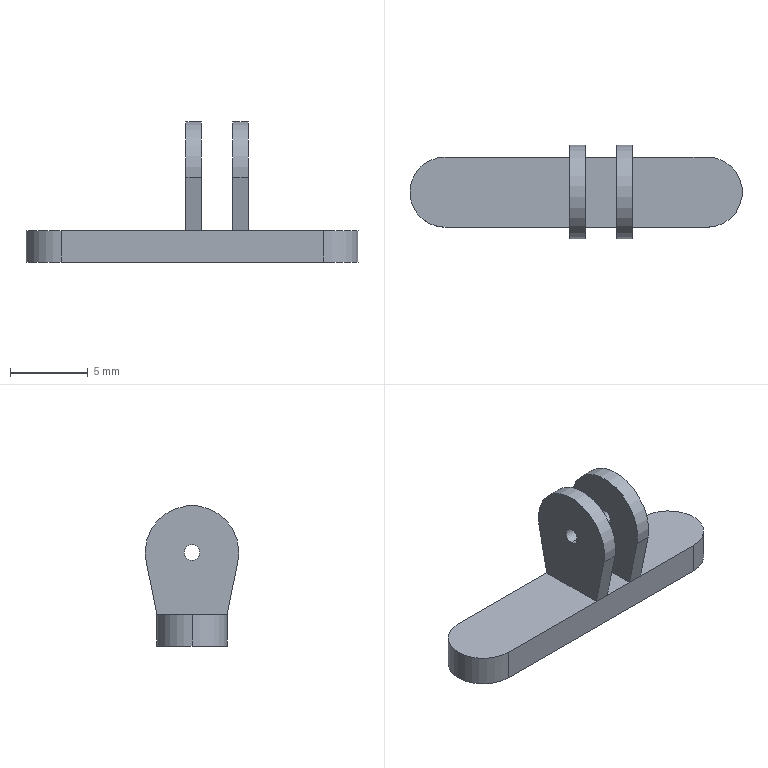Part | SolidWorks | features ICE 2, Extrusion 1 | 1 solid | 21 faces | box 21.3 x 6 x 9 mm | volume 252.148 mm3 | plane 12 | cylinder 9 | commonest cylinder face diameters 1 x4 4.5 x3 6 x2
STEP:
#1=CARTESIAN_POINT('',(8.,0.0009773,5.5));
#2=VERTEX_POINT('',#1);
#3=CARTESIAN_POINT('',(8.,0.0009773,6.5));
#4=VERTEX_POINT('',#3);
#5=CARTESIAN_POINT('',(8.,0.0009773,6.));
#6=DIRECTION('',(-1.,0.,0.));
#7=DIRECTION('',(0.,0.,1.));
#8=AXIS2_PLACEMENT_3D('',#5,#6,#7);
#9=CIRCLE('',#8,0.5);
#10=EDGE_CURVE('',#2,#4,#9,.T.);
#11=ORIENTED_EDGE('',*,*,#10,.T.);
#12=CARTESIAN_POINT('',(9.,0.0009773,6.5));
#13=VERTEX_POINT('',#12);
#14=CARTESIAN_POINT('',(8.,0.0009773,6.5));
#15=DIRECTION('',(1.,0.,0.));
#16=VECTOR('',#15,1000.);
#17=LINE('',#14,#16);
#18=EDGE_CURVE('',#4,#13,#17,.T.);
#19=ORIENTED_EDGE('',*,*,#18,.T.);
#20=CARTESIAN_POINT('',(9.,0.0009773,5.5));
#21=VERTEX_POINT('',#20);
#22=CARTESIAN_POINT('',(9.,0.0009773,6.));
#23=DIRECTION('',(-1.,0.,0.));
#24=DIRECTION('',(0.,0.,1.));
#25=AXIS2_PLACEMENT_3D('',#22,#23,#24);
#26=CIRCLE('',#25,0.5);
#27=EDGE_CURVE('',#21,#13,#26,.T.);
#28=ORIENTED_EDGE('',*,*,#27,.F.);
#29=CARTESIAN_POINT('',(8.,0.0009773,5.5));
#30=DIRECTION('',(1.,0.,0.));
#31=VECTOR('',#30,1000.);
#32=LINE('',#29,#31);
#33=EDGE_CURVE('',#2,#21,#32,.T.);
#34=ORIENTED_EDGE('',*,*,#33,.F.);
#35=EDGE_LOOP('',(#11,#19,#28,#34));
#36=FACE_OUTER_BOUND('',#35,.T.);
#37=CARTESIAN_POINT('',(8.,0.0009773,6.));
#38=DIRECTION('',(1.,0.,0.));
#39=DIRECTION('',(0.,0.,-1.));
#40=AXIS2_PLACEMENT_3D('',#37,#38,#39);
#41=CYLINDRICAL_SURFACE('',#40,0.5);
#42=ADVANCED_FACE('',(#36),#41,.F.);
#43=CARTESIAN_POINT('',(-2.25,0.,2.));
#44=VERTEX_POINT('',#43);
#45=CARTESIAN_POINT('',(0.,-2.25,2.));
#46=VERTEX_POINT('',#45);
#47=CARTESIAN_POINT('',(0.,0.,2.));
#48=DIRECTION('',(0.,0.,1.));
#49=DIRECTION('',(1.,0.,0.));
#50=AXIS2_PLACEMENT_3D('',#47,#48,#49);
#51=CIRCLE('',#50,2.25);
#52=EDGE_CURVE('',#44,#46,#51,.T.);
#53=ORIENTED_EDGE('',*,*,#52,.F.);
#54=CARTESIAN_POINT('',(-2.25,0.,0.));
#55=VERTEX_POINT('',#54);
#56=CARTESIAN_POINT('',(-2.25,0.,2.));
#57=DIRECTION('',(0.,0.,-1.));
#58=VECTOR('',#57,1000.);
#59=LINE('',#56,#58);
#60=EDGE_CURVE('',#44,#55,#59,.T.);
#61=ORIENTED_EDGE('',*,*,#60,.T.);
#62=CARTESIAN_POINT('',(0.,-2.25,0.));
#63=VERTEX_POINT('',#62);
#64=CARTESIAN_POINT('',(0.,0.,0.));
#65=DIRECTION('',(0.,0.,1.));
#66=DIRECTION('',(1.,0.,0.));
#67=AXIS2_PLACEMENT_3D('',#64,#65,#66);
#68=CIRCLE('',#67,2.25);
#69=EDGE_CURVE('',#55,#63,#68,.T.);
#70=ORIENTED_EDGE('',*,*,#69,.T.);
#71=CARTESIAN_POINT('',(0.,-2.25,2.));
#72=DIRECTION('',(0.,0.,-1.));
#73=VECTOR('',#72,1000.);
#74=LINE('',#71,#73);
#75=EDGE_CURVE('',#46,#63,#74,.T.);
#76=ORIENTED_EDGE('',*,*,#75,.F.);
#77=EDGE_LOOP('',(#53,#61,#70,#76));
#78=FACE_OUTER_BOUND('',#77,.T.);
#79=CARTESIAN_POINT('',(0.,0.,2.));
#80=DIRECTION('',(0.,0.,-1.));
#81=DIRECTION('',(-1.,0.,0.));
#82=AXIS2_PLACEMENT_3D('',#79,#80,#81);
#83=CYLINDRICAL_SURFACE('',#82,2.25);
#84=ADVANCED_FACE('',(#78),#83,.T.);
#85=CARTESIAN_POINT('',(11.,0.0009773,6.5));
#86=VERTEX_POINT('',#85);
#87=CARTESIAN_POINT('',(11.,0.0009773,5.5));
#88=VERTEX_POINT('',#87);
#89=CARTESIAN_POINT('',(11.,0.0009773,6.));
#90=DIRECTION('',(1.,0.,0.));
#91=DIRECTION('',(0.,0.,-1.));
#92=AXIS2_PLACEMENT_3D('',#89,#90,#91);
#93=CIRCLE('',#92,0.5);
#94=EDGE_CURVE('',#86,#88,#93,.T.);
#95=ORIENTED_EDGE('',*,*,#94,.F.);
#96=CARTESIAN_POINT('',(12.,0.0009773,6.5));
#97=VERTEX_POINT('',#96);
#98=CARTESIAN_POINT('',(8.,0.0009773,6.5));
#99=DIRECTION('',(1.,0.,0.));
#100=VECTOR('',#99,1000.);
#101=LINE('',#98,#100);
#102=EDGE_CURVE('',#86,#97,#101,.T.);
#103=ORIENTED_EDGE('',*,*,#102,.T.);
#104=CARTESIAN_POINT('',(12.,0.0009773,5.5));
#105=VERTEX_POINT('',#104);
#106=CARTESIAN_POINT('',(12.,0.0009773,6.));
#107=DIRECTION('',(-1.,0.,0.));
#108=DIRECTION('',(0.,0.,1.));
#109=AXIS2_PLACEMENT_3D('',#106,#107,#108);
#110=CIRCLE('',#109,0.5);
#111=EDGE_CURVE('',#105,#97,#110,.T.);
#112=ORIENTED_EDGE('',*,*,#111,.F.);
#113=CARTESIAN_POINT('',(8.,0.0009773,5.5));
#114=DIRECTION('',(1.,0.,0.));
#115=VECTOR('',#114,1000.);
#116=LINE('',#113,#115);
#117=EDGE_CURVE('',#88,#105,#116,.T.);
#118=ORIENTED_EDGE('',*,*,#117,.F.);
#119=EDGE_LOOP('',(#95,#103,#112,#118));
#120=FACE_OUTER_BOUND('',#119,.T.);
#121=CARTESIAN_POINT('',(8.,0.0009773,6.));
#122=DIRECTION('',(1.,0.,0.));
#123=DIRECTION('',(0.,0.,-1.));
#124=AXIS2_PLACEMENT_3D('',#121,#122,#123);
#125=CYLINDRICAL_SURFACE('',#124,0.5);
#126=ADVANCED_FACE('',(#120),#125,.F.);
#127=CARTESIAN_POINT('',(11.,2.25,2.));
#128=VERTEX_POINT('',#127);
#129=CARTESIAN_POINT('',(12.,2.25,2.));
#130=VERTEX_POINT('',#129);
#131=CARTESIAN_POINT('',(8.,2.25,2.));
#132=DIRECTION('',(1.,0.,0.));
#133=VECTOR('',#132,1000.);
#134=LINE('',#131,#133);
#135=EDGE_CURVE('',#128,#130,#134,.T.);
#136=ORIENTED_EDGE('',*,*,#135,.F.);
#137=CARTESIAN_POINT('',(11.,2.941,5.403));
#138=VERTEX_POINT('',#137);
#139=CARTESIAN_POINT('',(11.,2.25,2.));
#140=DIRECTION('',(0.,0.199,0.98));
#141=VECTOR('',#140,1000.);
#142=LINE('',#139,#141);
#143=EDGE_CURVE('',#128,#138,#142,.T.);
#144=ORIENTED_EDGE('',*,*,#143,.T.);
#145=CARTESIAN_POINT('',(12.,2.941,5.403));
#146=VERTEX_POINT('',#145);
#147=CARTESIAN_POINT('',(8.,2.941,5.403));
#148=DIRECTION('',(1.,0.,0.));
#149=VECTOR('',#148,1000.);
#150=LINE('',#147,#149);
#151=EDGE_CURVE('',#138,#146,#150,.T.);
#152=ORIENTED_EDGE('',*,*,#151,.T.);
#153=CARTESIAN_POINT('',(12.,2.25,2.));
#154=DIRECTION('',(0.,-0.199,-0.98));
#155=VECTOR('',#154,1000.);
#156=LINE('',#153,#155);
#157=EDGE_CURVE('',#146,#130,#156,.T.);
#158=ORIENTED_EDGE('',*,*,#157,.T.);
#159=EDGE_LOOP('',(#136,#144,#152,#158));
#160=FACE_OUTER_BOUND('',#159,.T.);
#161=CARTESIAN_POINT('',(8.,2.25,2.));
#162=DIRECTION('',(0.,-0.98,0.199));
#163=DIRECTION('',(0.,-0.199,-0.98));
#164=AXIS2_PLACEMENT_3D('',#161,#162,#163);
#165=PLANE('',#164);
#166=ADVANCED_FACE('',(#160),#165,.F.);
#167=CARTESIAN_POINT('',(11.,-2.939,5.404));
#168=VERTEX_POINT('',#167);
#169=CARTESIAN_POINT('',(12.,-2.939,5.404));
#170=VERTEX_POINT('',#169);
#171=CARTESIAN_POINT('',(8.,-2.939,5.404));
#172=DIRECTION('',(1.,0.,0.));
#173=VECTOR('',#172,1000.);
#174=LINE('',#171,#173);
#175=EDGE_CURVE('',#168,#170,#174,.T.);
#176=ORIENTED_EDGE('',*,*,#175,.F.);
#177=CARTESIAN_POINT('',(11.,-2.249,2.));
#178=VERTEX_POINT('',#177);
#179=CARTESIAN_POINT('',(11.,-2.249,2.));
#180=DIRECTION('',(0.,0.1987,-0.9801));
#181=VECTOR('',#180,1000.);
#182=LINE('',#179,#181);
#183=EDGE_CURVE('',#168,#178,#182,.T.);
#184=ORIENTED_EDGE('',*,*,#183,.T.);
#185=CARTESIAN_POINT('',(12.,-2.249,2.));
#186=VERTEX_POINT('',#185);
#187=CARTESIAN_POINT('',(8.,-2.249,2.));
#188=DIRECTION('',(1.,0.,0.));
#189=VECTOR('',#188,1000.);
#190=LINE('',#187,#189);
#191=EDGE_CURVE('',#178,#186,#190,.T.);
#192=ORIENTED_EDGE('',*,*,#191,.T.);
#193=CARTESIAN_POINT('',(12.,-2.249,2.));
#194=DIRECTION('',(0.,-0.1987,0.9801));
#195=VECTOR('',#194,1000.);
#196=LINE('',#193,#195);
#197=EDGE_CURVE('',#186,#170,#196,.T.);
#198=ORIENTED_EDGE('',*,*,#197,.T.);
#199=EDGE_LOOP('',(#176,#184,#192,#198));
#200=FACE_OUTER_BOUND('',#199,.T.);
#201=CARTESIAN_POINT('',(8.,-2.249,2.));
#202=DIRECTION('',(0.,0.9801,0.1987));
#203=DIRECTION('',(0.,-0.1987,0.9801));
#204=AXIS2_PLACEMENT_3D('',#201,#202,#203);
#205=PLANE('',#204);
#206=ADVANCED_FACE('',(#200),#205,.F.);
#207=CARTESIAN_POINT('',(8.,-2.939,5.404));
#208=VERTEX_POINT('',#207);
#209=CARTESIAN_POINT('',(9.,-2.939,5.404));
#210=VERTEX_POINT('',#209);
#211=CARTESIAN_POINT('',(8.,-2.939,5.404));
#212=DIRECTION('',(1.,0.,0.));
#213=VECTOR('',#212,1000.);
#214=LINE('',#211,#213);
#215=EDGE_CURVE('',#208,#210,#214,.T.);
#216=ORIENTED_EDGE('',*,*,#215,.T.);
#217=CARTESIAN_POINT('',(9.,2.941,5.403));
#218=VERTEX_POINT('',#217);
#219=CARTESIAN_POINT('',(9.,0.0009773,6.));
#220=DIRECTION('',(-1.,0.,0.));
#221=DIRECTION('',(0.,0.,1.));
#222=AXIS2_PLACEMENT_3D('',#219,#220,#221);
#223=CIRCLE('',#222,3.);
#224=EDGE_CURVE('',#210,#218,#223,.T.);
#225=ORIENTED_EDGE('',*,*,#224,.T.);
#226=CARTESIAN_POINT('',(8.,2.941,5.403));
#227=VERTEX_POINT('',#226);
#228=CARTESIAN_POINT('',(8.,2.941,5.403));
#229=DIRECTION('',(1.,0.,0.));
#230=VECTOR('',#229,1000.);
#231=LINE('',#228,#230);
#232=EDGE_CURVE('',#227,#218,#231,.T.);
#233=ORIENTED_EDGE('',*,*,#232,.F.);
#234=CARTESIAN_POINT('',(8.,0.0009773,6.));
#235=DIRECTION('',(-1.,0.,0.));
#236=DIRECTION('',(0.,0.,1.));
#237=AXIS2_PLACEMENT_3D('',#234,#235,#236);
#238=CIRCLE('',#237,3.);
#239=EDGE_CURVE('',#208,#227,#238,.T.);
#240=ORIENTED_EDGE('',*,*,#239,.F.);
#241=EDGE_LOOP('',(#216,#225,#233,#240));
#242=FACE_OUTER_BOUND('',#241,.T.);
#243=CARTESIAN_POINT('',(8.,0.0009773,6.));
#244=DIRECTION('',(1.,0.,0.));
#245=DIRECTION('',(0.,0.,-1.));
#246=AXIS2_PLACEMENT_3D('',#243,#244,#245);
#247=CYLINDRICAL_SURFACE('',#246,3.);
#248=ADVANCED_FACE('',(#242),#247,.T.);
#249=ORIENTED_EDGE('',*,*,#102,.F.);
#250=CARTESIAN_POINT('',(11.,0.0009773,6.));
#251=DIRECTION('',(1.,0.,0.));
#252=DIRECTION('',(0.,0.,-1.));
#253=AXIS2_PLACEMENT_3D('',#250,#251,#252);
#254=CIRCLE('',#253,0.5);
#255=EDGE_CURVE('',#88,#86,#254,.T.);
#256=ORIENTED_EDGE('',*,*,#255,.F.);
#257=ORIENTED_EDGE('',*,*,#117,.T.);
#258=CARTESIAN_POINT('',(12.,0.0009773,6.));
#259=DIRECTION('',(-1.,0.,0.));
#260=DIRECTION('',(0.,0.,1.));
#261=AXIS2_PLACEMENT_3D('',#258,#259,#260);
#262=CIRCLE('',#261,0.5);
#263=EDGE_CURVE('',#97,#105,#262,.T.);
#264=ORIENTED_EDGE('',*,*,#263,.F.);
#265=EDGE_LOOP('',(#249,#256,#257,#264));
#266=FACE_OUTER_BOUND('',#265,.T.);
#267=CARTESIAN_POINT('',(8.,0.0009773,6.));
#268=DIRECTION('',(1.,0.,0.));
#269=DIRECTION('',(0.,0.,-1.));
#270=AXIS2_PLACEMENT_3D('',#267,#268,#269);
#271=CYLINDRICAL_SURFACE('',#270,0.5);
#272=ADVANCED_FACE('',(#266),#271,.F.);
#273=CARTESIAN_POINT('',(16.8,-2.25,2.));
#274=VERTEX_POINT('',#273);
#275=CARTESIAN_POINT('',(0.,-2.25,2.));
#276=DIRECTION('',(1.,0.,0.));
#277=VECTOR('',#276,1000.);
#278=LINE('',#275,#277);
#279=EDGE_CURVE('',#46,#274,#278,.T.);
#280=ORIENTED_EDGE('',*,*,#279,.T.);
#281=CARTESIAN_POINT('',(16.8,2.25,2.));
#282=VERTEX_POINT('',#281);
#283=CARTESIAN_POINT('',(16.8,0.,2.));
#284=DIRECTION('',(0.,0.,1.));
#285=DIRECTION('',(1.,0.,0.));
#286=AXIS2_PLACEMENT_3D('',#283,#284,#285);
#287=CIRCLE('',#286,2.25);
#288=EDGE_CURVE('',#274,#282,#287,.T.);
#289=ORIENTED_EDGE('',*,*,#288,.T.);
#290=CARTESIAN_POINT('',(0.,2.25,2.));
#291=DIRECTION('',(-1.,0.,0.));
#292=VECTOR('',#291,1000.);
#293=LINE('',#290,#292);
#294=EDGE_CURVE('',#282,#130,#293,.T.);
#295=ORIENTED_EDGE('',*,*,#294,.T.);
#296=CARTESIAN_POINT('',(12.,2.25,2.));
#297=DIRECTION('',(0.,-1.,0.));
#298=VECTOR('',#297,1000.);
#299=LINE('',#296,#298);
#300=EDGE_CURVE('',#130,#186,#299,.T.);
#301=ORIENTED_EDGE('',*,*,#300,.T.);
#302=ORIENTED_EDGE('',*,*,#191,.F.);
#303=CARTESIAN_POINT('',(11.,-2.999,2.));
#304=DIRECTION('',(0.,1.,0.));
#305=VECTOR('',#304,1000.);
#306=LINE('',#303,#305);
#307=EDGE_CURVE('',#178,#128,#306,.T.);
#308=ORIENTED_EDGE('',*,*,#307,.T.);
#309=CARTESIAN_POINT('',(9.,2.25,2.));
#310=VERTEX_POINT('',#309);
#311=CARTESIAN_POINT('',(8.,2.25,2.));
#312=DIRECTION('',(1.,0.,0.));
#313=VECTOR('',#312,1000.);
#314=LINE('',#311,#313);
#315=EDGE_CURVE('',#310,#128,#314,.T.);
#316=ORIENTED_EDGE('',*,*,#315,.F.);
#317=CARTESIAN_POINT('',(9.,-2.249,2.));
#318=VERTEX_POINT('',#317);
#319=CARTESIAN_POINT('',(9.,-2.999,2.));
#320=DIRECTION('',(0.,1.,0.));
#321=VECTOR('',#320,1000.);
#322=LINE('',#319,#321);
#323=EDGE_CURVE('',#318,#310,#322,.T.);
#324=ORIENTED_EDGE('',*,*,#323,.F.);
#325=CARTESIAN_POINT('',(8.,-2.249,2.));
#326=VERTEX_POINT('',#325);
#327=CARTESIAN_POINT('',(8.,-2.249,2.));
#328=DIRECTION('',(1.,0.,0.));
#329=VECTOR('',#328,1000.);
#330=LINE('',#327,#329);
#331=EDGE_CURVE('',#326,#318,#330,.T.);
#332=ORIENTED_EDGE('',*,*,#331,.F.);
#333=CARTESIAN_POINT('',(8.,2.25,2.));
#334=VERTEX_POINT('',#333);
#335=CARTESIAN_POINT('',(8.,2.25,2.));
#336=DIRECTION('',(0.,-1.,0.));
#337=VECTOR('',#336,1000.);
#338=LINE('',#335,#337);
#339=EDGE_CURVE('',#334,#326,#338,.T.);
#340=ORIENTED_EDGE('',*,*,#339,.F.);
#341=CARTESIAN_POINT('',(0.,2.25,2.));
#342=VERTEX_POINT('',#341);
#343=CARTESIAN_POINT('',(0.,2.25,2.));
#344=DIRECTION('',(-1.,0.,0.));
#345=VECTOR('',#344,1000.);
#346=LINE('',#343,#345);
#347=EDGE_CURVE('',#334,#342,#346,.T.);
#348=ORIENTED_EDGE('',*,*,#347,.T.);
#349=CARTESIAN_POINT('',(0.,0.,2.));
#350=DIRECTION('',(0.,0.,1.));
#351=DIRECTION('',(1.,0.,0.));
#352=AXIS2_PLACEMENT_3D('',#349,#350,#351);
#353=CIRCLE('',#352,2.25);
#354=EDGE_CURVE('',#342,#44,#353,.T.);
#355=ORIENTED_EDGE('',*,*,#354,.T.);
#356=ORIENTED_EDGE('',*,*,#52,.T.);
#357=EDGE_LOOP('',(#280,#289,#295,#301,#302,#308,#316,#324,#332,#340,#348,#355,#356));
#358=FACE_OUTER_BOUND('',#357,.T.);
#359=CARTESIAN_POINT('',(0.,0.,2.));
#360=DIRECTION('',(0.,0.,1.));
#361=DIRECTION('',(1.,0.,0.));
#362=AXIS2_PLACEMENT_3D('',#359,#360,#361);
#363=PLANE('',#362);
#364=ADVANCED_FACE('',(#358),#363,.T.);
#365=ORIENTED_EDGE('',*,*,#60,.F.);
#366=ORIENTED_EDGE('',*,*,#354,.F.);
#367=CARTESIAN_POINT('',(0.,2.25,0.));
#368=VERTEX_POINT('',#367);
#369=CARTESIAN_POINT('',(0.,2.25,2.));
#370=DIRECTION('',(0.,0.,-1.));
#371=VECTOR('',#370,1000.);
#372=LINE('',#369,#371);
#373=EDGE_CURVE('',#342,#368,#372,.T.);
#374=ORIENTED_EDGE('',*,*,#373,.T.);
#375=CARTESIAN_POINT('',(0.,0.,0.));
#376=DIRECTION('',(0.,0.,1.));
#377=DIRECTION('',(1.,0.,0.));
#378=AXIS2_PLACEMENT_3D('',#375,#376,#377);
#379=CIRCLE('',#378,2.25);
#380=EDGE_CURVE('',#368,#55,#379,.T.);
#381=ORIENTED_EDGE('',*,*,#380,.T.);
#382=EDGE_LOOP('',(#365,#366,#374,#381));
#383=FACE_OUTER_BOUND('',#382,.T.);
#384=CARTESIAN_POINT('',(0.,0.,2.));
#385=DIRECTION('',(0.,0.,-1.));
#386=DIRECTION('',(-1.,0.,0.));
#387=AXIS2_PLACEMENT_3D('',#384,#385,#386);
#388=CYLINDRICAL_SURFACE('',#387,2.25);
#389=ADVANCED_FACE('',(#383),#388,.T.);
#390=CARTESIAN_POINT('',(16.8,-2.25,0.));
#391=VERTEX_POINT('',#390);
#392=CARTESIAN_POINT('',(0.,-2.25,0.));
#393=DIRECTION('',(1.,0.,0.));
#394=VECTOR('',#393,1000.);
#395=LINE('',#392,#394);
#396=EDGE_CURVE('',#63,#391,#395,.T.);
#397=ORIENTED_EDGE('',*,*,#396,.T.);
#398=CARTESIAN_POINT('',(16.8,-2.25,2.));
#399=DIRECTION('',(0.,0.,-1.));
#400=VECTOR('',#399,1000.);
#401=LINE('',#398,#400);
#402=EDGE_CURVE('',#274,#391,#401,.T.);
#403=ORIENTED_EDGE('',*,*,#402,.F.);
#404=ORIENTED_EDGE('',*,*,#279,.F.);
#405=ORIENTED_EDGE('',*,*,#75,.T.);
#406=EDGE_LOOP('',(#397,#403,#404,#405));
#407=FACE_OUTER_BOUND('',#406,.T.);
#408=CARTESIAN_POINT('',(0.,-2.25,2.));
#409=DIRECTION('',(0.,1.,0.));
#410=DIRECTION('',(0.,0.,1.));
#411=AXIS2_PLACEMENT_3D('',#408,#409,#410);
#412=PLANE('',#411);
#413=ADVANCED_FACE('',(#407),#412,.F.);
#414=CARTESIAN_POINT('',(16.8,2.25,0.));
#415=VERTEX_POINT('',#414);
#416=CARTESIAN_POINT('',(16.8,0.,0.));
#417=DIRECTION('',(0.,0.,1.));
#418=DIRECTION('',(1.,0.,0.));
#419=AXIS2_PLACEMENT_3D('',#416,#417,#418);
#420=CIRCLE('',#419,2.25);
#421=EDGE_CURVE('',#391,#415,#420,.T.);
#422=ORIENTED_EDGE('',*,*,#421,.T.);
#423=CARTESIAN_POINT('',(16.8,2.25,2.));
#424=DIRECTION('',(0.,0.,-1.));
#425=VECTOR('',#424,1000.);
#426=LINE('',#423,#425);
#427=EDGE_CURVE('',#282,#415,#426,.T.);
#428=ORIENTED_EDGE('',*,*,#427,.F.);
#429=ORIENTED_EDGE('',*,*,#288,.F.);
#430=ORIENTED_EDGE('',*,*,#402,.T.);
#431=EDGE_LOOP('',(#422,#428,#429,#430));
#432=FACE_OUTER_BOUND('',#431,.T.);
#433=CARTESIAN_POINT('',(16.8,0.,2.));
#434=DIRECTION('',(0.,0.,-1.));
#435=DIRECTION('',(-1.,0.,0.));
#436=AXIS2_PLACEMENT_3D('',#433,#434,#435);
#437=CYLINDRICAL_SURFACE('',#436,2.25);
#438=ADVANCED_FACE('',(#432),#437,.T.);
#439=CARTESIAN_POINT('',(0.,2.25,0.));
#440=DIRECTION('',(-1.,0.,0.));
#441=VECTOR('',#440,1000.);
#442=LINE('',#439,#441);
#443=EDGE_CURVE('',#415,#368,#442,.T.);
#444=ORIENTED_EDGE('',*,*,#443,.T.);
#445=ORIENTED_EDGE('',*,*,#373,.F.);
#446=ORIENTED_EDGE('',*,*,#347,.F.);
#447=CARTESIAN_POINT('',(8.,2.25,2.));
#448=DIRECTION('',(1.,0.,0.));
#449=VECTOR('',#448,1000.);
#450=LINE('',#447,#449);
#451=EDGE_CURVE('',#334,#310,#450,.T.);
#452=ORIENTED_EDGE('',*,*,#451,.T.);
#453=ORIENTED_EDGE('',*,*,#315,.T.);
#454=ORIENTED_EDGE('',*,*,#135,.T.);
#455=ORIENTED_EDGE('',*,*,#294,.F.);
#456=ORIENTED_EDGE('',*,*,#427,.T.);
#457=EDGE_LOOP('',(#444,#445,#446,#452,#453,#454,#455,#456));
#458=FACE_OUTER_BOUND('',#457,.T.);
#459=CARTESIAN_POINT('',(0.,2.25,2.));
#460=DIRECTION('',(0.,-1.,0.));
#461=DIRECTION('',(0.,0.,-1.));
#462=AXIS2_PLACEMENT_3D('',#459,#460,#461);
#463=PLANE('',#462);
#464=ADVANCED_FACE('',(#458),#463,.F.);
#465=ORIENTED_EDGE('',*,*,#380,.F.);
#466=ORIENTED_EDGE('',*,*,#443,.F.);
#467=ORIENTED_EDGE('',*,*,#421,.F.);
#468=ORIENTED_EDGE('',*,*,#396,.F.);
#469=ORIENTED_EDGE('',*,*,#69,.F.);
#470=EDGE_LOOP('',(#465,#466,#467,#468,#469));
#471=FACE_OUTER_BOUND('',#470,.T.);
#472=CARTESIAN_POINT('',(0.,0.,0.));
#473=DIRECTION('',(0.,0.,1.));
#474=DIRECTION('',(1.,0.,0.));
#475=AXIS2_PLACEMENT_3D('',#472,#473,#474);
#476=PLANE('',#475);
#477=ADVANCED_FACE('',(#471),#476,.F.);
#478=CARTESIAN_POINT('',(8.,2.25,2.));
#479=DIRECTION('',(0.,-0.199,-0.98));
#480=VECTOR('',#479,1000.);
#481=LINE('',#478,#480);
#482=EDGE_CURVE('',#227,#334,#481,.T.);
#483=ORIENTED_EDGE('',*,*,#482,.T.);
#484=ORIENTED_EDGE('',*,*,#339,.T.);
#485=CARTESIAN_POINT('',(8.,-2.249,2.));
#486=DIRECTION('',(0.,-0.1987,0.9801));
#487=VECTOR('',#486,1000.);
#488=LINE('',#485,#487);
#489=EDGE_CURVE('',#326,#208,#488,.T.);
#490=ORIENTED_EDGE('',*,*,#489,.T.);
#491=ORIENTED_EDGE('',*,*,#239,.T.);
#492=EDGE_LOOP('',(#483,#484,#490,#491));
#493=FACE_OUTER_BOUND('',#492,.T.);
#494=ORIENTED_EDGE('',*,*,#10,.F.);
#495=CARTESIAN_POINT('',(8.,0.0009773,6.));
#496=DIRECTION('',(-1.,0.,0.));
#497=DIRECTION('',(0.,0.,1.));
#498=AXIS2_PLACEMENT_3D('',#495,#496,#497);
#499=CIRCLE('',#498,0.5);
#500=EDGE_CURVE('',#4,#2,#499,.T.);
#501=ORIENTED_EDGE('',*,*,#500,.F.);
#502=EDGE_LOOP('',(#494,#501));
#503=FACE_BOUND('',#502,.T.);
#504=CARTESIAN_POINT('',(8.,0.0009773,6.));
#505=DIRECTION('',(-1.,0.,0.));
#506=DIRECTION('',(0.,0.,1.));
#507=AXIS2_PLACEMENT_3D('',#504,#505,#506);
#508=PLANE('',#507);
#509=ADVANCED_FACE('',(#493,#503),#508,.T.);
#510=ORIENTED_EDGE('',*,*,#157,.F.);
#511=CARTESIAN_POINT('',(12.,0.0009773,6.));
#512=DIRECTION('',(-1.,0.,0.));
#513=DIRECTION('',(0.,0.,1.));
#514=AXIS2_PLACEMENT_3D('',#511,#512,#513);
#515=CIRCLE('',#514,3.);
#516=EDGE_CURVE('',#170,#146,#515,.T.);
#517=ORIENTED_EDGE('',*,*,#516,.F.);
#518=ORIENTED_EDGE('',*,*,#197,.F.);
#519=ORIENTED_EDGE('',*,*,#300,.F.);
#520=EDGE_LOOP('',(#510,#517,#518,#519));
#521=FACE_OUTER_BOUND('',#520,.T.);
#522=ORIENTED_EDGE('',*,*,#111,.T.);
#523=ORIENTED_EDGE('',*,*,#263,.T.);
#524=EDGE_LOOP('',(#522,#523));
#525=FACE_BOUND('',#524,.T.);
#526=CARTESIAN_POINT('',(12.,0.0009773,6.));
#527=DIRECTION('',(-1.,0.,0.));
#528=DIRECTION('',(0.,0.,1.));
#529=AXIS2_PLACEMENT_3D('',#526,#527,#528);
#530=PLANE('',#529);
#531=ADVANCED_FACE('',(#521,#525),#530,.F.);
#532=ORIENTED_EDGE('',*,*,#232,.T.);
#533=CARTESIAN_POINT('',(9.,2.25,2.));
#534=DIRECTION('',(0.,-0.199,-0.98));
#535=VECTOR('',#534,1000.);
#536=LINE('',#533,#535);
#537=EDGE_CURVE('',#218,#310,#536,.T.);
#538=ORIENTED_EDGE('',*,*,#537,.T.);
#539=ORIENTED_EDGE('',*,*,#451,.F.);
#540=ORIENTED_EDGE('',*,*,#482,.F.);
#541=EDGE_LOOP('',(#532,#538,#539,#540));
#542=FACE_OUTER_BOUND('',#541,.T.);
#543=CARTESIAN_POINT('',(8.,2.25,2.));
#544=DIRECTION('',(0.,-0.98,0.199));
#545=DIRECTION('',(0.,-0.199,-0.98));
#546=AXIS2_PLACEMENT_3D('',#543,#544,#545);
#547=PLANE('',#546);
#548=ADVANCED_FACE('',(#542),#547,.F.);
#549=ORIENTED_EDGE('',*,*,#331,.T.);
#550=CARTESIAN_POINT('',(9.,-2.249,2.));
#551=DIRECTION('',(0.,-0.1987,0.9801));
#552=VECTOR('',#551,1000.);
#553=LINE('',#550,#552);
#554=EDGE_CURVE('',#318,#210,#553,.T.);
#555=ORIENTED_EDGE('',*,*,#554,.T.);
#556=ORIENTED_EDGE('',*,*,#215,.F.);
#557=ORIENTED_EDGE('',*,*,#489,.F.);
#558=EDGE_LOOP('',(#549,#555,#556,#557));
#559=FACE_OUTER_BOUND('',#558,.T.);
#560=CARTESIAN_POINT('',(8.,-2.249,2.));
#561=DIRECTION('',(0.,0.9801,0.1987));
#562=DIRECTION('',(0.,-0.1987,0.9801));
#563=AXIS2_PLACEMENT_3D('',#560,#561,#562);
#564=PLANE('',#563);
#565=ADVANCED_FACE('',(#559),#564,.F.);
#566=ORIENTED_EDGE('',*,*,#151,.F.);
#567=CARTESIAN_POINT('',(11.,0.0009773,6.));
#568=DIRECTION('',(1.,0.,0.));
#569=DIRECTION('',(0.,0.,-1.));
#570=AXIS2_PLACEMENT_3D('',#567,#568,#569);
#571=CIRCLE('',#570,3.);
#572=EDGE_CURVE('',#138,#168,#571,.T.);
#573=ORIENTED_EDGE('',*,*,#572,.T.);
#574=ORIENTED_EDGE('',*,*,#175,.T.);
#575=ORIENTED_EDGE('',*,*,#516,.T.);
#576=EDGE_LOOP('',(#566,#573,#574,#575));
#577=FACE_OUTER_BOUND('',#576,.T.);
#578=CARTESIAN_POINT('',(8.,0.0009773,6.));
#579=DIRECTION('',(1.,0.,0.));
#580=DIRECTION('',(0.,0.,-1.));
#581=AXIS2_PLACEMENT_3D('',#578,#579,#580);
#582=CYLINDRICAL_SURFACE('',#581,3.);
#583=ADVANCED_FACE('',(#577),#582,.T.);
#584=ORIENTED_EDGE('',*,*,#18,.F.);
#585=ORIENTED_EDGE('',*,*,#500,.T.);
#586=ORIENTED_EDGE('',*,*,#33,.T.);
#587=CARTESIAN_POINT('',(9.,0.0009773,6.));
#588=DIRECTION('',(-1.,0.,0.));
#589=DIRECTION('',(0.,0.,1.));
#590=AXIS2_PLACEMENT_3D('',#587,#588,#589);
#591=CIRCLE('',#590,0.5);
#592=EDGE_CURVE('',#13,#21,#591,.T.);
#593=ORIENTED_EDGE('',*,*,#592,.F.);
#594=EDGE_LOOP('',(#584,#585,#586,#593));
#595=FACE_OUTER_BOUND('',#594,.T.);
#596=CARTESIAN_POINT('',(8.,0.0009773,6.));
#597=DIRECTION('',(1.,0.,0.));
#598=DIRECTION('',(0.,0.,-1.));
#599=AXIS2_PLACEMENT_3D('',#596,#597,#598);
#600=CYLINDRICAL_SURFACE('',#599,0.5);
#601=ADVANCED_FACE('',(#595),#600,.F.);
#602=ORIENTED_EDGE('',*,*,#255,.T.);
#603=ORIENTED_EDGE('',*,*,#94,.T.);
#604=EDGE_LOOP('',(#602,#603));
#605=FACE_BOUND('',#604,.T.);
#606=ORIENTED_EDGE('',*,*,#572,.F.);
#607=ORIENTED_EDGE('',*,*,#143,.F.);
#608=ORIENTED_EDGE('',*,*,#307,.F.);
#609=ORIENTED_EDGE('',*,*,#183,.F.);
#610=EDGE_LOOP('',(#606,#607,#608,#609));
#611=FACE_OUTER_BOUND('',#610,.T.);
#612=CARTESIAN_POINT('',(11.,-2.999,10.093));
#613=DIRECTION('',(1.,0.,0.));
#614=DIRECTION('',(0.,0.,-1.));
#615=AXIS2_PLACEMENT_3D('',#612,#613,#614);
#616=PLANE('',#615);
#617=ADVANCED_FACE('',(#605,#611),#616,.F.);
#618=ORIENTED_EDGE('',*,*,#27,.T.);
#619=ORIENTED_EDGE('',*,*,#592,.T.);
#620=EDGE_LOOP('',(#618,#619));
#621=FACE_BOUND('',#620,.T.);
#622=ORIENTED_EDGE('',*,*,#224,.F.);
#623=ORIENTED_EDGE('',*,*,#554,.F.);
#624=ORIENTED_EDGE('',*,*,#323,.T.);
#625=ORIENTED_EDGE('',*,*,#537,.F.);
#626=EDGE_LOOP('',(#622,#623,#624,#625));
#627=FACE_OUTER_BOUND('',#626,.T.);
#628=CARTESIAN_POINT('',(9.,-2.999,2.));
#629=DIRECTION('',(-1.,0.,0.));
#630=DIRECTION('',(0.,0.,1.));
#631=AXIS2_PLACEMENT_3D('',#628,#629,#630);
#632=PLANE('',#631);
#633=ADVANCED_FACE('',(#621,#627),#632,.F.);
#634=CLOSED_SHELL('',(#42,#84,#126,#166,#206,#248,#272,#364,#389,#413,#438,#464,#477,#509,#531,#548,#565,#583,#601,#617,#633));
#635=MANIFOLD_SOLID_BREP('',#634);
#636=CARTESIAN_POINT('',(0.,0.,0.));
#637=DIRECTION('',(0.,0.,1.));
#638=DIRECTION('',(1.,0.,0.));
#639=AXIS2_PLACEMENT_3D('',#636,#637,#638);
#640=(LENGTH_UNIT()NAMED_UNIT(*)SI_UNIT(.MILLI.,.METRE.));
#641=UNCERTAINTY_MEASURE_WITH_UNIT(LENGTH_MEASURE(0.00001),#640,'','');
#642=(NAMED_UNIT(*)PLANE_ANGLE_UNIT()SI_UNIT($,.RADIAN.));
#643=(NAMED_UNIT(*)SI_UNIT($,.STERADIAN.)SOLID_ANGLE_UNIT());
#644=(GEOMETRIC_REPRESENTATION_CONTEXT(3)GLOBAL_UNCERTAINTY_ASSIGNED_CONTEXT((#641))GLOBAL_UNIT_ASSIGNED_CONTEXT((#640,#642,#643))REPRESENTATION_CONTEXT('',''));
#645=ADVANCED_BREP_SHAPE_REPRESENTATION('',(#635,#639),#644);